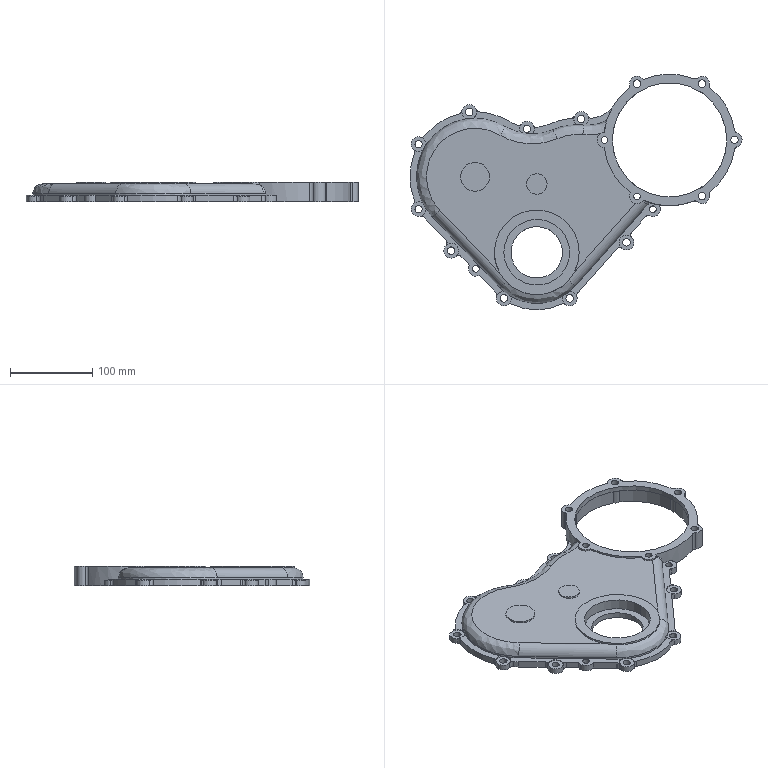Part | SolidWorks | features BaseBody 1 | 1 solid | 248 faces | box 403.298 x 286.452 x 24 mm | volume 403922 mm3 | cylinder 169 | plane 48 | spline 22 | cone 9 | commonest cylinder face diameters 18 x51 8 x42 9 x26 142 x7 160 x7 103 x4